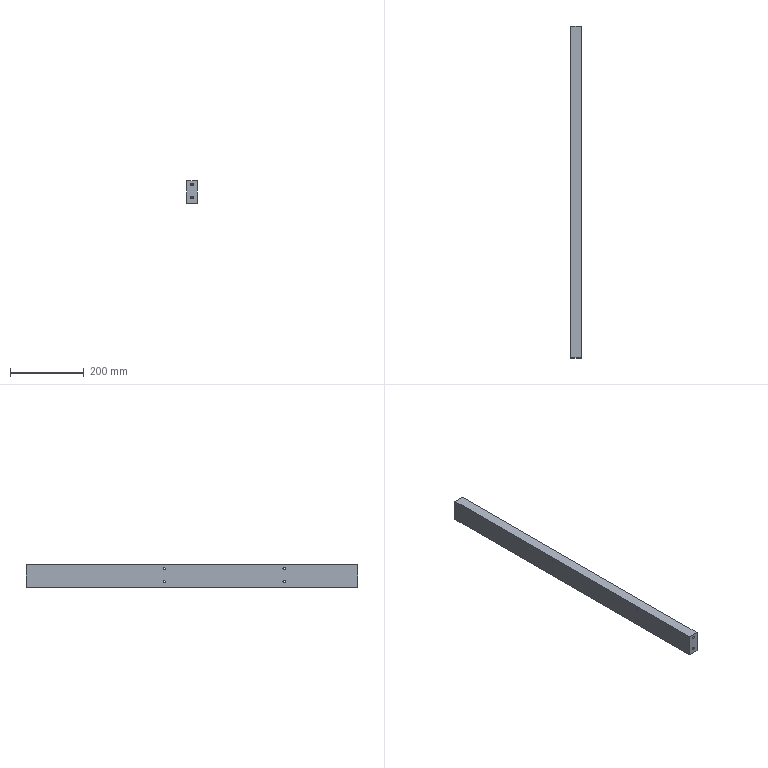Part | STEP file | PN_0054 (guide rail fixed plate) | 1 solid | 78 faces | box 28 x 900 x 60 mm | volume 1504828 mm3 | cylinder 40 | cone 32 | plane 6 | commonest cylinder face diameters 3.3 x24 6.8 x12 5 x4